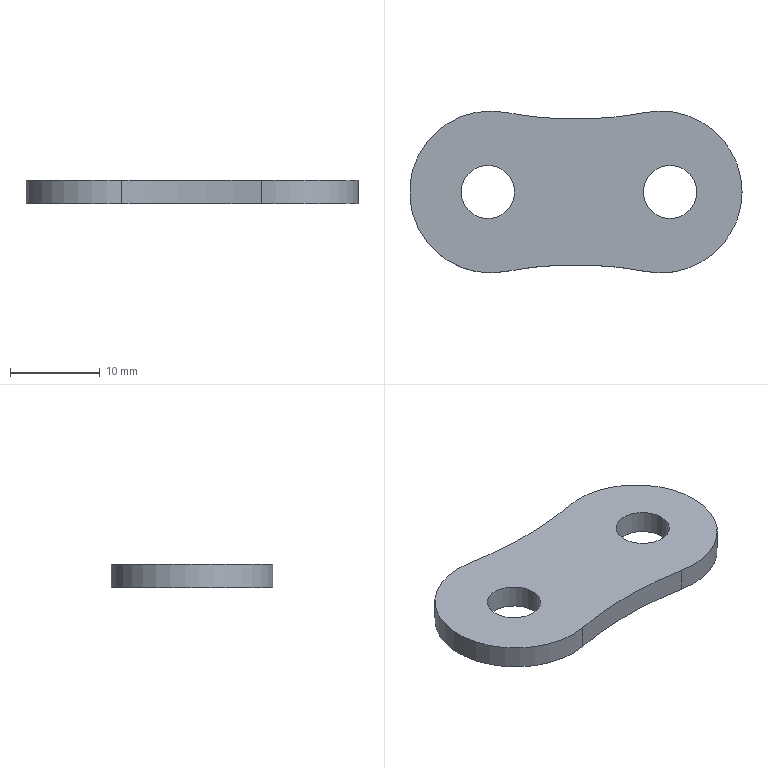Part | SolidWorks | features MoveFace 2, BaseBody 1 | 1 solid | 11 faces | box 37.13 x 18.08 x 2.59 mm | volume 1358 mm3 | cylinder 9 | plane 2 | commonest cylinder face diameters 5.96 x4 18.08 x3 83.184 x2
STEP:
#1=CARTESIAN_POINT('',(-98.03,-121.026,-11.465));
#2=VERTEX_POINT('',#1);
#3=CARTESIAN_POINT('',(-92.07,-121.026,-11.465));
#4=VERTEX_POINT('',#3);
#5=CARTESIAN_POINT('',(-95.05,-121.026,-11.465));
#6=DIRECTION('',(0.,0.,1.));
#7=DIRECTION('',(1.,0.,0.));
#8=AXIS2_PLACEMENT_3D('',#5,#6,#7);
#9=CIRCLE('',#8,2.98);
#10=EDGE_CURVE('',#2,#4,#9,.T.);
#11=ORIENTED_EDGE('',*,*,#10,.F.);
#12=CARTESIAN_POINT('',(-98.03,-121.026,-8.875));
#13=VERTEX_POINT('',#12);
#14=CARTESIAN_POINT('',(-98.03,-121.026,-11.465));
#15=DIRECTION('',(0.,0.,1.));
#16=VECTOR('',#15,1000.);
#17=LINE('',#14,#16);
#18=EDGE_CURVE('',#2,#13,#17,.T.);
#19=ORIENTED_EDGE('',*,*,#18,.T.);
#20=CARTESIAN_POINT('',(-92.07,-121.026,-8.875));
#21=VERTEX_POINT('',#20);
#22=CARTESIAN_POINT('',(-95.05,-121.026,-8.875));
#23=DIRECTION('',(0.,0.,-1.));
#24=DIRECTION('',(1.,0.,0.));
#25=AXIS2_PLACEMENT_3D('',#22,#23,#24);
#26=CIRCLE('',#25,2.98);
#27=EDGE_CURVE('',#21,#13,#26,.T.);
#28=ORIENTED_EDGE('',*,*,#27,.F.);
#29=CARTESIAN_POINT('',(-92.07,-121.026,-11.465));
#30=DIRECTION('',(0.,0.,1.));
#31=VECTOR('',#30,1000.);
#32=LINE('',#29,#31);
#33=EDGE_CURVE('',#4,#21,#32,.T.);
#34=ORIENTED_EDGE('',*,*,#33,.F.);
#35=EDGE_LOOP('',(#11,#19,#28,#34));
#36=FACE_OUTER_BOUND('',#35,.T.);
#37=CARTESIAN_POINT('',(-95.05,-121.026,-11.465));
#38=DIRECTION('',(0.,0.,1.));
#39=DIRECTION('',(1.,0.,0.));
#40=AXIS2_PLACEMENT_3D('',#37,#38,#39);
#41=CYLINDRICAL_SURFACE('',#40,2.98);
#42=ADVANCED_FACE('',(#36),#41,.F.);
#43=CARTESIAN_POINT('',(-66.66,-121.026,-11.465));
#44=VERTEX_POINT('',#43);
#45=CARTESIAN_POINT('',(-77.4,-129.905,-11.465));
#46=VERTEX_POINT('',#45);
#47=CARTESIAN_POINT('',(-75.7,-121.026,-11.465));
#48=DIRECTION('',(0.,0.,-1.));
#49=DIRECTION('',(1.,0.,0.));
#50=AXIS2_PLACEMENT_3D('',#47,#48,#49);
#51=CIRCLE('',#50,9.04);
#52=EDGE_CURVE('',#44,#46,#51,.T.);
#53=ORIENTED_EDGE('',*,*,#52,.F.);
#54=CARTESIAN_POINT('',(-66.66,-121.026,-8.875));
#55=VERTEX_POINT('',#54);
#56=CARTESIAN_POINT('',(-66.66,-121.026,-11.465));
#57=DIRECTION('',(0.,0.,1.));
#58=VECTOR('',#57,1000.);
#59=LINE('',#56,#58);
#60=EDGE_CURVE('',#44,#55,#59,.T.);
#61=ORIENTED_EDGE('',*,*,#60,.T.);
#62=CARTESIAN_POINT('',(-77.4,-129.905,-8.875));
#63=VERTEX_POINT('',#62);
#64=CARTESIAN_POINT('',(-75.7,-121.026,-8.875));
#65=DIRECTION('',(0.,0.,-1.));
#66=DIRECTION('',(1.,0.,0.));
#67=AXIS2_PLACEMENT_3D('',#64,#65,#66);
#68=CIRCLE('',#67,9.04);
#69=EDGE_CURVE('',#55,#63,#68,.T.);
#70=ORIENTED_EDGE('',*,*,#69,.T.);
#71=CARTESIAN_POINT('',(-77.4,-129.905,-11.465));
#72=DIRECTION('',(0.,0.,-1.));
#73=VECTOR('',#72,1000.);
#74=LINE('',#71,#73);
#75=EDGE_CURVE('',#63,#46,#74,.T.);
#76=ORIENTED_EDGE('',*,*,#75,.T.);
#77=EDGE_LOOP('',(#53,#61,#70,#76));
#78=FACE_OUTER_BOUND('',#77,.T.);
#79=CARTESIAN_POINT('',(-75.7,-121.026,-11.465));
#80=DIRECTION('',(0.,0.,1.));
#81=DIRECTION('',(1.,0.,0.));
#82=AXIS2_PLACEMENT_3D('',#79,#80,#81);
#83=CYLINDRICAL_SURFACE('',#82,9.04);
#84=ADVANCED_FACE('',(#78),#83,.T.);
#85=CARTESIAN_POINT('',(-77.68,-121.026,-11.465));
#86=VERTEX_POINT('',#85);
#87=CARTESIAN_POINT('',(-71.72,-121.026,-11.465));
#88=VERTEX_POINT('',#87);
#89=CARTESIAN_POINT('',(-74.7,-121.026,-11.465));
#90=DIRECTION('',(0.,0.,1.));
#91=DIRECTION('',(1.,0.,0.));
#92=AXIS2_PLACEMENT_3D('',#89,#90,#91);
#93=CIRCLE('',#92,2.98);
#94=EDGE_CURVE('',#86,#88,#93,.T.);
#95=ORIENTED_EDGE('',*,*,#94,.F.);
#96=CARTESIAN_POINT('',(-77.68,-121.026,-8.875));
#97=VERTEX_POINT('',#96);
#98=CARTESIAN_POINT('',(-77.68,-121.026,-11.465));
#99=DIRECTION('',(0.,0.,1.));
#100=VECTOR('',#99,1000.);
#101=LINE('',#98,#100);
#102=EDGE_CURVE('',#86,#97,#101,.T.);
#103=ORIENTED_EDGE('',*,*,#102,.T.);
#104=CARTESIAN_POINT('',(-71.72,-121.026,-8.875));
#105=VERTEX_POINT('',#104);
#106=CARTESIAN_POINT('',(-74.7,-121.026,-8.875));
#107=DIRECTION('',(0.,0.,-1.));
#108=DIRECTION('',(1.,0.,0.));
#109=AXIS2_PLACEMENT_3D('',#106,#107,#108);
#110=CIRCLE('',#109,2.98);
#111=EDGE_CURVE('',#105,#97,#110,.T.);
#112=ORIENTED_EDGE('',*,*,#111,.F.);
#113=CARTESIAN_POINT('',(-71.72,-121.026,-11.465));
#114=DIRECTION('',(0.,0.,1.));
#115=VECTOR('',#114,1000.);
#116=LINE('',#113,#115);
#117=EDGE_CURVE('',#88,#105,#116,.T.);
#118=ORIENTED_EDGE('',*,*,#117,.F.);
#119=EDGE_LOOP('',(#95,#103,#112,#118));
#120=FACE_OUTER_BOUND('',#119,.T.);
#121=CARTESIAN_POINT('',(-74.7,-121.026,-11.465));
#122=DIRECTION('',(0.,0.,1.));
#123=DIRECTION('',(1.,0.,0.));
#124=AXIS2_PLACEMENT_3D('',#121,#122,#123);
#125=CYLINDRICAL_SURFACE('',#124,2.98);
#126=ADVANCED_FACE('',(#120),#125,.F.);
#127=CARTESIAN_POINT('',(-95.05,-121.026,-11.465));
#128=DIRECTION('',(0.,0.,1.));
#129=DIRECTION('',(1.,0.,0.));
#130=AXIS2_PLACEMENT_3D('',#127,#128,#129);
#131=CIRCLE('',#130,2.98);
#132=EDGE_CURVE('',#4,#2,#131,.T.);
#133=ORIENTED_EDGE('',*,*,#132,.T.);
#134=ORIENTED_EDGE('',*,*,#10,.T.);
#135=EDGE_LOOP('',(#133,#134));
#136=FACE_BOUND('',#135,.T.);
#137=CARTESIAN_POINT('',(-77.4,-112.148,-11.465));
#138=VERTEX_POINT('',#137);
#139=CARTESIAN_POINT('',(-75.7,-121.026,-11.465));
#140=DIRECTION('',(0.,0.,-1.));
#141=DIRECTION('',(1.,0.,0.));
#142=AXIS2_PLACEMENT_3D('',#139,#140,#141);
#143=CIRCLE('',#142,9.04);
#144=EDGE_CURVE('',#138,#44,#143,.T.);
#145=ORIENTED_EDGE('',*,*,#144,.T.);
#146=ORIENTED_EDGE('',*,*,#52,.T.);
#147=CARTESIAN_POINT('',(-93.049,-129.905,-11.465));
#148=VERTEX_POINT('',#147);
#149=CARTESIAN_POINT('',(-85.225,-170.754,-11.465));
#150=DIRECTION('',(0.,0.,1.));
#151=DIRECTION('',(1.,0.,0.));
#152=AXIS2_PLACEMENT_3D('',#149,#150,#151);
#153=CIRCLE('',#152,41.592);
#154=EDGE_CURVE('',#46,#148,#153,.T.);
#155=ORIENTED_EDGE('',*,*,#154,.T.);
#156=CARTESIAN_POINT('',(-93.049,-112.148,-11.465));
#157=VERTEX_POINT('',#156);
#158=CARTESIAN_POINT('',(-94.75,-121.026,-11.465));
#159=DIRECTION('',(0.,0.,-1.));
#160=DIRECTION('',(1.,0.,0.));
#161=AXIS2_PLACEMENT_3D('',#158,#159,#160);
#162=CIRCLE('',#161,9.04);
#163=EDGE_CURVE('',#148,#157,#162,.T.);
#164=ORIENTED_EDGE('',*,*,#163,.T.);
#165=CARTESIAN_POINT('',(-85.225,-71.298,-11.465));
#166=DIRECTION('',(0.,0.,1.));
#167=DIRECTION('',(1.,0.,0.));
#168=AXIS2_PLACEMENT_3D('',#165,#166,#167);
#169=CIRCLE('',#168,41.592);
#170=EDGE_CURVE('',#157,#138,#169,.T.);
#171=ORIENTED_EDGE('',*,*,#170,.T.);
#172=EDGE_LOOP('',(#145,#146,#155,#164,#171));
#173=FACE_OUTER_BOUND('',#172,.T.);
#174=CARTESIAN_POINT('',(-74.7,-121.026,-11.465));
#175=DIRECTION('',(0.,0.,1.));
#176=DIRECTION('',(1.,0.,0.));
#177=AXIS2_PLACEMENT_3D('',#174,#175,#176);
#178=CIRCLE('',#177,2.98);
#179=EDGE_CURVE('',#88,#86,#178,.T.);
#180=ORIENTED_EDGE('',*,*,#179,.T.);
#181=ORIENTED_EDGE('',*,*,#94,.T.);
#182=EDGE_LOOP('',(#180,#181));
#183=FACE_BOUND('',#182,.T.);
#184=CARTESIAN_POINT('',(-89.987,-145.89,-11.465));
#185=DIRECTION('',(0.,0.,-1.));
#186=DIRECTION('',(-1.,0.,0.));
#187=AXIS2_PLACEMENT_3D('',#184,#185,#186);
#188=PLANE('',#187);
#189=ADVANCED_FACE('',(#136,#173,#183),#188,.T.);
#190=ORIENTED_EDGE('',*,*,#18,.F.);
#191=ORIENTED_EDGE('',*,*,#132,.F.);
#192=ORIENTED_EDGE('',*,*,#33,.T.);
#193=CARTESIAN_POINT('',(-95.05,-121.026,-8.875));
#194=DIRECTION('',(0.,0.,-1.));
#195=DIRECTION('',(1.,0.,0.));
#196=AXIS2_PLACEMENT_3D('',#193,#194,#195);
#197=CIRCLE('',#196,2.98);
#198=EDGE_CURVE('',#13,#21,#197,.T.);
#199=ORIENTED_EDGE('',*,*,#198,.F.);
#200=EDGE_LOOP('',(#190,#191,#192,#199));
#201=FACE_OUTER_BOUND('',#200,.T.);
#202=CARTESIAN_POINT('',(-95.05,-121.026,-11.465));
#203=DIRECTION('',(0.,0.,1.));
#204=DIRECTION('',(1.,0.,0.));
#205=AXIS2_PLACEMENT_3D('',#202,#203,#204);
#206=CYLINDRICAL_SURFACE('',#205,2.98);
#207=ADVANCED_FACE('',(#201),#206,.F.);
#208=ORIENTED_EDGE('',*,*,#60,.F.);
#209=ORIENTED_EDGE('',*,*,#144,.F.);
#210=CARTESIAN_POINT('',(-77.4,-112.148,-8.875));
#211=VERTEX_POINT('',#210);
#212=CARTESIAN_POINT('',(-77.4,-112.148,-11.465));
#213=DIRECTION('',(0.,0.,1.));
#214=VECTOR('',#213,1000.);
#215=LINE('',#212,#214);
#216=EDGE_CURVE('',#138,#211,#215,.T.);
#217=ORIENTED_EDGE('',*,*,#216,.T.);
#218=CARTESIAN_POINT('',(-75.7,-121.026,-8.875));
#219=DIRECTION('',(0.,0.,-1.));
#220=DIRECTION('',(1.,0.,0.));
#221=AXIS2_PLACEMENT_3D('',#218,#219,#220);
#222=CIRCLE('',#221,9.04);
#223=EDGE_CURVE('',#211,#55,#222,.T.);
#224=ORIENTED_EDGE('',*,*,#223,.T.);
#225=EDGE_LOOP('',(#208,#209,#217,#224));
#226=FACE_OUTER_BOUND('',#225,.T.);
#227=CARTESIAN_POINT('',(-75.7,-121.026,-11.465));
#228=DIRECTION('',(0.,0.,1.));
#229=DIRECTION('',(1.,0.,0.));
#230=AXIS2_PLACEMENT_3D('',#227,#228,#229);
#231=CYLINDRICAL_SURFACE('',#230,9.04);
#232=ADVANCED_FACE('',(#226),#231,.T.);
#233=ORIENTED_EDGE('',*,*,#216,.F.);
#234=ORIENTED_EDGE('',*,*,#170,.F.);
#235=CARTESIAN_POINT('',(-93.049,-112.148,-8.875));
#236=VERTEX_POINT('',#235);
#237=CARTESIAN_POINT('',(-93.049,-112.148,-11.465));
#238=DIRECTION('',(0.,0.,-1.));
#239=VECTOR('',#238,1000.);
#240=LINE('',#237,#239);
#241=EDGE_CURVE('',#236,#157,#240,.T.);
#242=ORIENTED_EDGE('',*,*,#241,.F.);
#243=CARTESIAN_POINT('',(-85.225,-71.298,-8.875));
#244=DIRECTION('',(0.,0.,-1.));
#245=DIRECTION('',(1.,0.,0.));
#246=AXIS2_PLACEMENT_3D('',#243,#244,#245);
#247=CIRCLE('',#246,41.592);
#248=EDGE_CURVE('',#211,#236,#247,.T.);
#249=ORIENTED_EDGE('',*,*,#248,.F.);
#250=EDGE_LOOP('',(#233,#234,#242,#249));
#251=FACE_OUTER_BOUND('',#250,.T.);
#252=CARTESIAN_POINT('',(-85.225,-71.298,-11.465));
#253=DIRECTION('',(0.,0.,1.));
#254=DIRECTION('',(1.,0.,0.));
#255=AXIS2_PLACEMENT_3D('',#252,#253,#254);
#256=CYLINDRICAL_SURFACE('',#255,41.592);
#257=ADVANCED_FACE('',(#251),#256,.F.);
#258=ORIENTED_EDGE('',*,*,#163,.F.);
#259=CARTESIAN_POINT('',(-93.049,-129.905,-8.875));
#260=VERTEX_POINT('',#259);
#261=CARTESIAN_POINT('',(-93.049,-129.905,-11.465));
#262=DIRECTION('',(0.,0.,1.));
#263=VECTOR('',#262,1000.);
#264=LINE('',#261,#263);
#265=EDGE_CURVE('',#148,#260,#264,.T.);
#266=ORIENTED_EDGE('',*,*,#265,.T.);
#267=CARTESIAN_POINT('',(-94.75,-121.026,-8.875));
#268=DIRECTION('',(0.,0.,-1.));
#269=DIRECTION('',(1.,0.,0.));
#270=AXIS2_PLACEMENT_3D('',#267,#268,#269);
#271=CIRCLE('',#270,9.04);
#272=EDGE_CURVE('',#260,#236,#271,.T.);
#273=ORIENTED_EDGE('',*,*,#272,.T.);
#274=ORIENTED_EDGE('',*,*,#241,.T.);
#275=EDGE_LOOP('',(#258,#266,#273,#274));
#276=FACE_OUTER_BOUND('',#275,.T.);
#277=CARTESIAN_POINT('',(-94.75,-121.026,-11.465));
#278=DIRECTION('',(0.,0.,1.));
#279=DIRECTION('',(1.,0.,0.));
#280=AXIS2_PLACEMENT_3D('',#277,#278,#279);
#281=CYLINDRICAL_SURFACE('',#280,9.04);
#282=ADVANCED_FACE('',(#276),#281,.T.);
#283=ORIENTED_EDGE('',*,*,#265,.F.);
#284=ORIENTED_EDGE('',*,*,#154,.F.);
#285=ORIENTED_EDGE('',*,*,#75,.F.);
#286=CARTESIAN_POINT('',(-85.225,-170.754,-8.875));
#287=DIRECTION('',(0.,0.,-1.));
#288=DIRECTION('',(1.,0.,0.));
#289=AXIS2_PLACEMENT_3D('',#286,#287,#288);
#290=CIRCLE('',#289,41.592);
#291=EDGE_CURVE('',#260,#63,#290,.T.);
#292=ORIENTED_EDGE('',*,*,#291,.F.);
#293=EDGE_LOOP('',(#283,#284,#285,#292));
#294=FACE_OUTER_BOUND('',#293,.T.);
#295=CARTESIAN_POINT('',(-85.225,-170.754,-11.465));
#296=DIRECTION('',(0.,0.,1.));
#297=DIRECTION('',(1.,0.,0.));
#298=AXIS2_PLACEMENT_3D('',#295,#296,#297);
#299=CYLINDRICAL_SURFACE('',#298,41.592);
#300=ADVANCED_FACE('',(#294),#299,.F.);
#301=ORIENTED_EDGE('',*,*,#102,.F.);
#302=ORIENTED_EDGE('',*,*,#179,.F.);
#303=ORIENTED_EDGE('',*,*,#117,.T.);
#304=CARTESIAN_POINT('',(-74.7,-121.026,-8.875));
#305=DIRECTION('',(0.,0.,-1.));
#306=DIRECTION('',(1.,0.,0.));
#307=AXIS2_PLACEMENT_3D('',#304,#305,#306);
#308=CIRCLE('',#307,2.98);
#309=EDGE_CURVE('',#97,#105,#308,.T.);
#310=ORIENTED_EDGE('',*,*,#309,.F.);
#311=EDGE_LOOP('',(#301,#302,#303,#310));
#312=FACE_OUTER_BOUND('',#311,.T.);
#313=CARTESIAN_POINT('',(-74.7,-121.026,-11.465));
#314=DIRECTION('',(0.,0.,1.));
#315=DIRECTION('',(1.,0.,0.));
#316=AXIS2_PLACEMENT_3D('',#313,#314,#315);
#317=CYLINDRICAL_SURFACE('',#316,2.98);
#318=ADVANCED_FACE('',(#312),#317,.F.);
#319=ORIENTED_EDGE('',*,*,#27,.T.);
#320=ORIENTED_EDGE('',*,*,#198,.T.);
#321=EDGE_LOOP('',(#319,#320));
#322=FACE_BOUND('',#321,.T.);
#323=ORIENTED_EDGE('',*,*,#111,.T.);
#324=ORIENTED_EDGE('',*,*,#309,.T.);
#325=EDGE_LOOP('',(#323,#324));
#326=FACE_BOUND('',#325,.T.);
#327=ORIENTED_EDGE('',*,*,#223,.F.);
#328=ORIENTED_EDGE('',*,*,#248,.T.);
#329=ORIENTED_EDGE('',*,*,#272,.F.);
#330=ORIENTED_EDGE('',*,*,#291,.T.);
#331=ORIENTED_EDGE('',*,*,#69,.F.);
#332=EDGE_LOOP('',(#327,#328,#329,#330,#331));
#333=FACE_OUTER_BOUND('',#332,.T.);
#334=CARTESIAN_POINT('',(-89.987,-145.89,-8.875));
#335=DIRECTION('',(0.,0.,-1.));
#336=DIRECTION('',(-1.,0.,0.));
#337=AXIS2_PLACEMENT_3D('',#334,#335,#336);
#338=PLANE('',#337);
#339=ADVANCED_FACE('',(#322,#326,#333),#338,.F.);
#340=CLOSED_SHELL('',(#42,#84,#126,#189,#207,#232,#257,#282,#300,#318,#339));
#341=MANIFOLD_SOLID_BREP('',#340);
#342=CARTESIAN_POINT('',(0.,0.,0.));
#343=DIRECTION('',(0.,0.,1.));
#344=DIRECTION('',(1.,0.,0.));
#345=AXIS2_PLACEMENT_3D('',#342,#343,#344);
#346=(LENGTH_UNIT()NAMED_UNIT(*)SI_UNIT(.MILLI.,.METRE.));
#347=UNCERTAINTY_MEASURE_WITH_UNIT(LENGTH_MEASURE(0.00001),#346,'','');
#348=(NAMED_UNIT(*)PLANE_ANGLE_UNIT()SI_UNIT($,.RADIAN.));
#349=(NAMED_UNIT(*)SI_UNIT($,.STERADIAN.)SOLID_ANGLE_UNIT());
#350=(GEOMETRIC_REPRESENTATION_CONTEXT(3)GLOBAL_UNCERTAINTY_ASSIGNED_CONTEXT((#347))GLOBAL_UNIT_ASSIGNED_CONTEXT((#346,#348,#349))REPRESENTATION_CONTEXT('',''));
#351=ADVANCED_BREP_SHAPE_REPRESENTATION('',(#341,#345),#350);